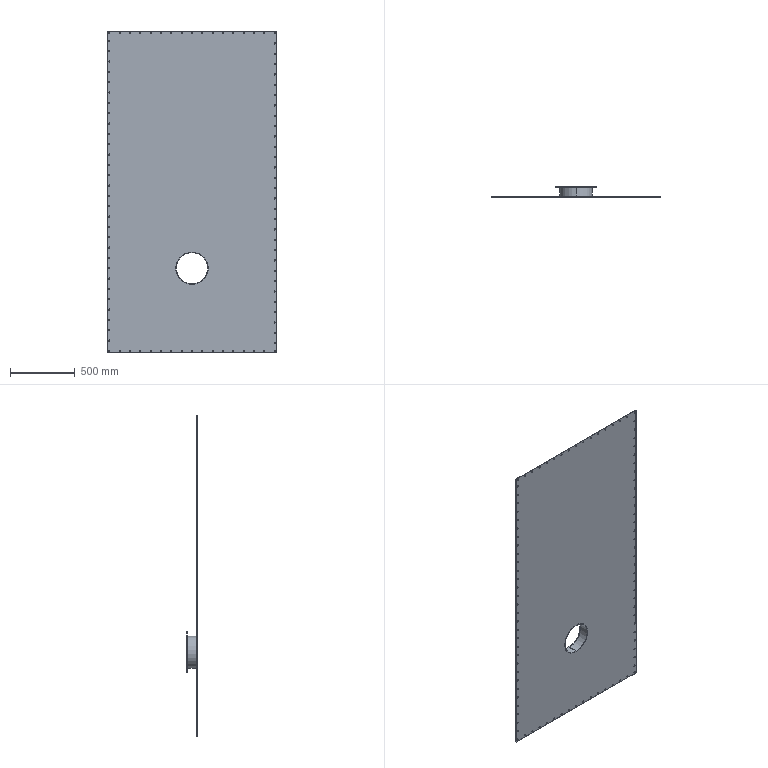Part | SolidWorks | 3 solids | 226 faces | box 1310 x 80 x 2490 mm | volume 13192841 mm3 | cylinder 214 | plane 12 | commonest cylinder face diameters 10 x188 6 x16 250 x6 242 x2 320 x2